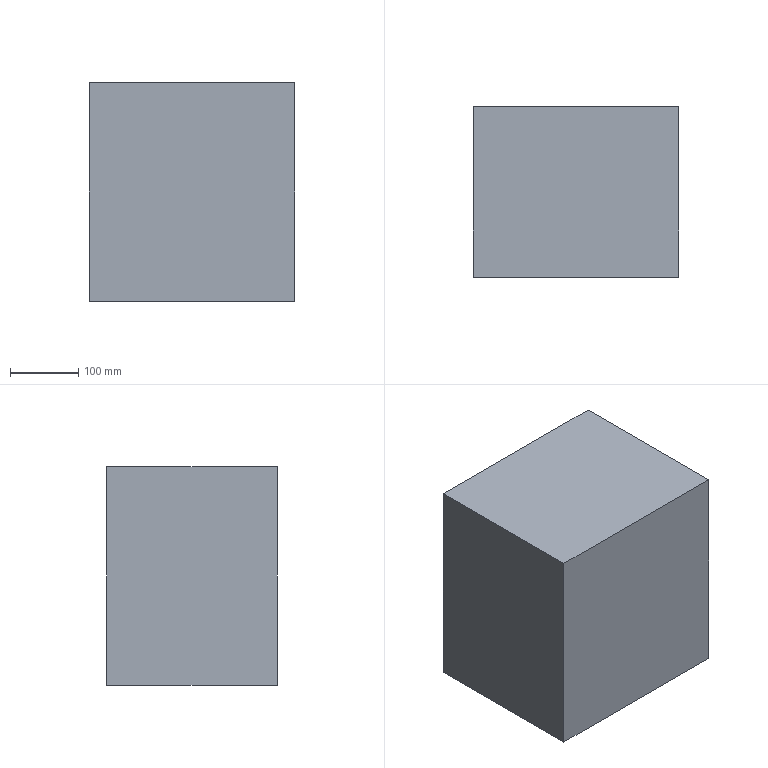Part | SolidWorks | features Extrusion 1 | 1 solid | 6 faces | box 300 x 250 x 320 mm | volume 24000000 mm3 | plane 6
STEP:
#1=CARTESIAN_POINT('',(150.,0.,160.));
#2=VERTEX_POINT('',#1);
#3=CARTESIAN_POINT('',(150.,0.,-160.));
#4=VERTEX_POINT('',#3);
#5=CARTESIAN_POINT('',(150.,0.,-160.));
#6=DIRECTION('',(0.,0.,-1.));
#7=VECTOR('',#6,1000.);
#8=LINE('',#5,#7);
#9=EDGE_CURVE('',#2,#4,#8,.T.);
#10=ORIENTED_EDGE('',*,*,#9,.T.);
#11=CARTESIAN_POINT('',(150.,250.,-160.));
#12=VERTEX_POINT('',#11);
#13=CARTESIAN_POINT('',(150.,250.,-160.));
#14=DIRECTION('',(0.,-1.,0.));
#15=VECTOR('',#14,1000.);
#16=LINE('',#13,#15);
#17=EDGE_CURVE('',#12,#4,#16,.T.);
#18=ORIENTED_EDGE('',*,*,#17,.F.);
#19=CARTESIAN_POINT('',(150.,250.,160.));
#20=VERTEX_POINT('',#19);
#21=CARTESIAN_POINT('',(150.,250.,-160.));
#22=DIRECTION('',(0.,0.,-1.));
#23=VECTOR('',#22,1000.);
#24=LINE('',#21,#23);
#25=EDGE_CURVE('',#20,#12,#24,.T.);
#26=ORIENTED_EDGE('',*,*,#25,.F.);
#27=CARTESIAN_POINT('',(150.,250.,160.));
#28=DIRECTION('',(0.,-1.,0.));
#29=VECTOR('',#28,1000.);
#30=LINE('',#27,#29);
#31=EDGE_CURVE('',#20,#2,#30,.T.);
#32=ORIENTED_EDGE('',*,*,#31,.T.);
#33=EDGE_LOOP('',(#10,#18,#26,#32));
#34=FACE_OUTER_BOUND('',#33,.T.);
#35=CARTESIAN_POINT('',(150.,250.,-160.));
#36=DIRECTION('',(-1.,0.,0.));
#37=DIRECTION('',(0.,0.,1.));
#38=AXIS2_PLACEMENT_3D('',#35,#36,#37);
#39=PLANE('',#38);
#40=ADVANCED_FACE('',(#34),#39,.F.);
#41=CARTESIAN_POINT('',(-150.,0.,-160.));
#42=VERTEX_POINT('',#41);
#43=CARTESIAN_POINT('',(-150.,0.,-160.));
#44=DIRECTION('',(-1.,0.,0.));
#45=VECTOR('',#44,1000.);
#46=LINE('',#43,#45);
#47=EDGE_CURVE('',#4,#42,#46,.T.);
#48=ORIENTED_EDGE('',*,*,#47,.T.);
#49=CARTESIAN_POINT('',(-150.,250.,-160.));
#50=VERTEX_POINT('',#49);
#51=CARTESIAN_POINT('',(-150.,250.,-160.));
#52=DIRECTION('',(0.,-1.,0.));
#53=VECTOR('',#52,1000.);
#54=LINE('',#51,#53);
#55=EDGE_CURVE('',#50,#42,#54,.T.);
#56=ORIENTED_EDGE('',*,*,#55,.F.);
#57=CARTESIAN_POINT('',(-150.,250.,-160.));
#58=DIRECTION('',(-1.,0.,0.));
#59=VECTOR('',#58,1000.);
#60=LINE('',#57,#59);
#61=EDGE_CURVE('',#12,#50,#60,.T.);
#62=ORIENTED_EDGE('',*,*,#61,.F.);
#63=ORIENTED_EDGE('',*,*,#17,.T.);
#64=EDGE_LOOP('',(#48,#56,#62,#63));
#65=FACE_OUTER_BOUND('',#64,.T.);
#66=CARTESIAN_POINT('',(-150.,250.,-160.));
#67=DIRECTION('',(0.,0.,1.));
#68=DIRECTION('',(1.,0.,0.));
#69=AXIS2_PLACEMENT_3D('',#66,#67,#68);
#70=PLANE('',#69);
#71=ADVANCED_FACE('',(#65),#70,.F.);
#72=CARTESIAN_POINT('',(-150.,0.,160.));
#73=VERTEX_POINT('',#72);
#74=CARTESIAN_POINT('',(-150.,0.,-160.));
#75=DIRECTION('',(0.,0.,1.));
#76=VECTOR('',#75,1000.);
#77=LINE('',#74,#76);
#78=EDGE_CURVE('',#42,#73,#77,.T.);
#79=ORIENTED_EDGE('',*,*,#78,.T.);
#80=CARTESIAN_POINT('',(-150.,250.,160.));
#81=VERTEX_POINT('',#80);
#82=CARTESIAN_POINT('',(-150.,250.,160.));
#83=DIRECTION('',(0.,-1.,0.));
#84=VECTOR('',#83,1000.);
#85=LINE('',#82,#84);
#86=EDGE_CURVE('',#81,#73,#85,.T.);
#87=ORIENTED_EDGE('',*,*,#86,.F.);
#88=CARTESIAN_POINT('',(-150.,250.,-160.));
#89=DIRECTION('',(0.,0.,1.));
#90=VECTOR('',#89,1000.);
#91=LINE('',#88,#90);
#92=EDGE_CURVE('',#50,#81,#91,.T.);
#93=ORIENTED_EDGE('',*,*,#92,.F.);
#94=ORIENTED_EDGE('',*,*,#55,.T.);
#95=EDGE_LOOP('',(#79,#87,#93,#94));
#96=FACE_OUTER_BOUND('',#95,.T.);
#97=CARTESIAN_POINT('',(-150.,250.,-160.));
#98=DIRECTION('',(1.,0.,0.));
#99=DIRECTION('',(0.,0.,-1.));
#100=AXIS2_PLACEMENT_3D('',#97,#98,#99);
#101=PLANE('',#100);
#102=ADVANCED_FACE('',(#96),#101,.F.);
#103=CARTESIAN_POINT('',(-150.,0.,160.));
#104=DIRECTION('',(1.,0.,0.));
#105=VECTOR('',#104,1000.);
#106=LINE('',#103,#105);
#107=EDGE_CURVE('',#73,#2,#106,.T.);
#108=ORIENTED_EDGE('',*,*,#107,.T.);
#109=ORIENTED_EDGE('',*,*,#31,.F.);
#110=CARTESIAN_POINT('',(-150.,250.,160.));
#111=DIRECTION('',(1.,0.,0.));
#112=VECTOR('',#111,1000.);
#113=LINE('',#110,#112);
#114=EDGE_CURVE('',#81,#20,#113,.T.);
#115=ORIENTED_EDGE('',*,*,#114,.F.);
#116=ORIENTED_EDGE('',*,*,#86,.T.);
#117=EDGE_LOOP('',(#108,#109,#115,#116));
#118=FACE_OUTER_BOUND('',#117,.T.);
#119=CARTESIAN_POINT('',(-150.,250.,160.));
#120=DIRECTION('',(0.,0.,-1.));
#121=DIRECTION('',(-1.,0.,0.));
#122=AXIS2_PLACEMENT_3D('',#119,#120,#121);
#123=PLANE('',#122);
#124=ADVANCED_FACE('',(#118),#123,.F.);
#125=ORIENTED_EDGE('',*,*,#25,.T.);
#126=ORIENTED_EDGE('',*,*,#61,.T.);
#127=ORIENTED_EDGE('',*,*,#92,.T.);
#128=ORIENTED_EDGE('',*,*,#114,.T.);
#129=EDGE_LOOP('',(#125,#126,#127,#128));
#130=FACE_OUTER_BOUND('',#129,.T.);
#131=CARTESIAN_POINT('',(0.,250.,0.));
#132=DIRECTION('',(0.,1.,0.));
#133=DIRECTION('',(0.,0.,1.));
#134=AXIS2_PLACEMENT_3D('',#131,#132,#133);
#135=PLANE('',#134);
#136=ADVANCED_FACE('',(#130),#135,.T.);
#137=ORIENTED_EDGE('',*,*,#9,.F.);
#138=ORIENTED_EDGE('',*,*,#107,.F.);
#139=ORIENTED_EDGE('',*,*,#78,.F.);
#140=ORIENTED_EDGE('',*,*,#47,.F.);
#141=EDGE_LOOP('',(#137,#138,#139,#140));
#142=FACE_OUTER_BOUND('',#141,.T.);
#143=CARTESIAN_POINT('',(0.,0.,0.));
#144=DIRECTION('',(0.,1.,0.));
#145=DIRECTION('',(0.,0.,1.));
#146=AXIS2_PLACEMENT_3D('',#143,#144,#145);
#147=PLANE('',#146);
#148=ADVANCED_FACE('',(#142),#147,.F.);
#149=CLOSED_SHELL('',(#40,#71,#102,#124,#136,#148));
#150=MANIFOLD_SOLID_BREP('',#149);
#151=CARTESIAN_POINT('',(0.,0.,0.));
#152=DIRECTION('',(0.,0.,1.));
#153=DIRECTION('',(1.,0.,0.));
#154=AXIS2_PLACEMENT_3D('',#151,#152,#153);
#155=(LENGTH_UNIT()NAMED_UNIT(*)SI_UNIT(.MILLI.,.METRE.));
#156=UNCERTAINTY_MEASURE_WITH_UNIT(LENGTH_MEASURE(0.00001),#155,'','');
#157=(NAMED_UNIT(*)PLANE_ANGLE_UNIT()SI_UNIT($,.RADIAN.));
#158=(NAMED_UNIT(*)SI_UNIT($,.STERADIAN.)SOLID_ANGLE_UNIT());
#159=(GEOMETRIC_REPRESENTATION_CONTEXT(3)GLOBAL_UNCERTAINTY_ASSIGNED_CONTEXT((#156))GLOBAL_UNIT_ASSIGNED_CONTEXT((#155,#157,#158))REPRESENTATION_CONTEXT('',''));
#160=ADVANCED_BREP_SHAPE_REPRESENTATION('',(#150,#154),#159);